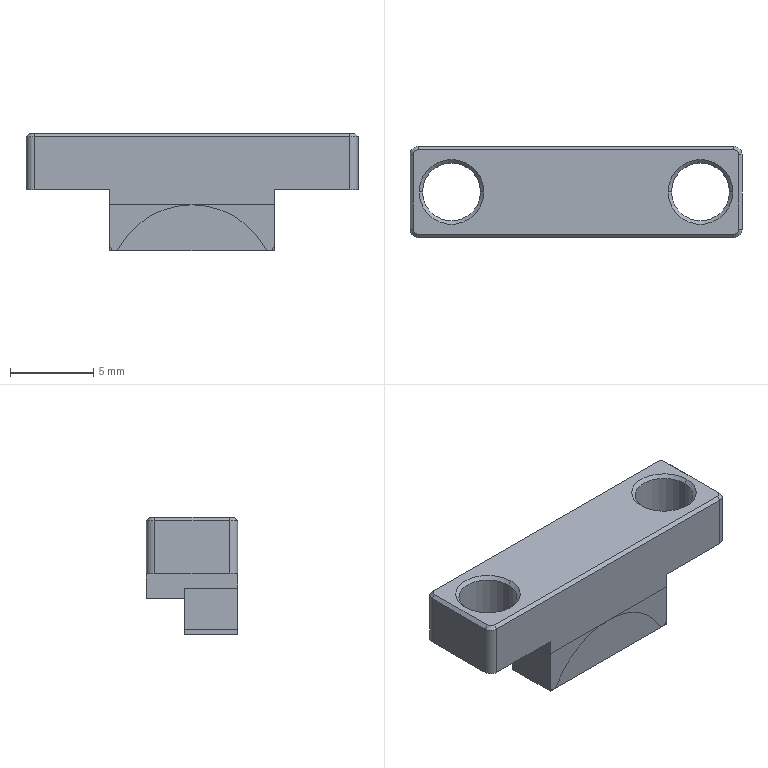NC program | NX | posted with a generic post | part box 20 x 5.5 x 7.057 mm
Whole program:
N10 G17 G21 G94 G90
(FLOOR_WALL_COPY_COPY , TOOL : D63)
N12 T03 M6
N14 G54
N16 G17 G0 G90 X44.499 Y0. B0. C0. S6500 M3
N18 G43 Z30. H3
N20 Z5.
N22 G94 G1 Z2. F1250.
N24 X41.499
N26 X-41.499
N28 X-44.499
N30 Z5.
N32 G0 Z30.
N34 X44.499
N36 Z4.
N38 G1 Z1.
N40 X41.499
N42 X-41.499
N44 X-44.499
N46 Z4.
N48 G0 Z30.
N50 X44.499
N52 Z3.
N54 G1 Z0.
N56 X41.499
N58 X-41.499
N60 X-44.499
N62 Z3.
N64 G0 Z30.
N66 M5
(FLOOR_WALL , TOOL : D6JING)
N68 T16 M6
N70 G54
N72 G17 G0 G90 X2.078 Y-8.75 B0. C0. S9500 M3
N74 G43 Z30. H16
N76 Z-0.377
N78 G94 G1 X0.52 Y-6.05 F1000.
N80 G3 X0. Y-5.75 R0.6
N82 G1 X-9.5 F2500.
N84 G2 X-13. Y-2.25 R3.5
N86 G1 Y2.25
N88 G2 X-9.5 Y5.75 R3.5
N90 G1 X-8.05
N92 Y-3.55
N94 X8.05
N96 Y5.75
N98 X9.5
N100 G2 X13. Y2.25 R3.5
N102 G1 Y-2.25
N104 G2 X9.5 Y-5.75 R3.5
N106 G1 X0.
N108 G3 X-0.52 Y-6.05 R0.6
N110 G1 X-2.078 Y-8.75
N112 G0 X2.078 Z-0.797
N114 G1 X0.52 Y-6.05 F1000.
N116 G3 X0. Y-5.75 R0.6
N118 G1 X-9.5 F2500.
N120 G2 X-13. Y-2.25 R3.5
N122 G1 Y2.25
N124 G2 X-9.5 Y5.75 R3.5
N126 G1 X-8.05
N128 Y-3.55
N130 X8.05
N132 Y5.75
N134 X9.5
N136 G2 X13. Y2.25 R3.5
N138 G1 Y-2.25
N140 G2 X9.5 Y-5.75 R3.5
N142 G1 X0.
N144 G3 X-0.52 Y-6.05 R0.6
N146 G1 X-2.078 Y-8.75
N148 G0 X2.078 Z-1.217
N150 G1 X0.52 Y-6.05 F1000.
N152 G3 X0. Y-5.75 R0.6
N154 G1 X-9.5 F2500.
N156 G2 X-13. Y-2.25 R3.5
N158 G1 Y2.25
N160 G2 X-9.5 Y5.75 R3.5
N162 G1 X-8.05
N164 Y-3.55
N166 X8.05
N168 Y5.75
N170 X9.5
N172 G2 X13. Y2.25 R3.5
N174 G1 Y-2.25
N176 G2 X9.5 Y-5.75 R3.5
N178 G1 X0.
N180 G3 X-0.52 Y-6.05 R0.6
N182 G1 X-2.078 Y-8.75
N184 G0 X2.078 Z-1.637
N186 G1 X0.52 Y-6.05 F1000.
N188 G3 X0. Y-5.75 R0.6
N190 G1 X-9.5 F2500.
N192 G2 X-13. Y-2.25 R3.5
N194 G1 Y2.25
N196 G2 X-9.5 Y5.75 R3.5
N198 G1 X-8.05
N200 Y-3.55
N202 X8.05
N204 Y5.75
N206 X9.5
N208 G2 X13. Y2.25 R3.5
N210 G1 Y-2.25
N212 G2 X9.5 Y-5.75 R3.5
N214 G1 X0.
N216 G3 X-0.52 Y-6.05 R0.6
N218 G1 X-2.078 Y-8.75
N220 G0 X2.078 Z-2.057
N222 G1 X0.52 Y-6.05 F1000.
N224 G3 X0. Y-5.75 R0.6
N226 G1 X-9.5 F2500.
N228 G2 X-13. Y-2.25 R3.5
N230 G1 Y2.25
N232 G2 X-9.5 Y5.75 R3.5
N234 G1 X-8.05
N236 Y-3.55
N238 X8.05
N240 Y5.75
N242 X9.5
N244 G2 X13. Y2.25 R3.5
N246 G1 Y-2.25
N248 G2 X9.5 Y-5.75 R3.5
N250 G1 X0.
N252 G3 X-0.52 Y-6.05 R0.6
N254 G1 X-2.078 Y-8.75
N256 G0 Z30.
N258 X-16. Y-2.078
N260 Z-2.557
N262 G1 X-13.3 Y-0.52 F1000.
N264 G3 X-13. Y0. R0.6
N266 G1 Y2.25 F2500.
N268 G2 X-9.5 Y5.75 R3.5
N270 G1 X-8.05
N272 Y-5.75
N274 X-9.5
N276 G2 X-13. Y-2.25 R3.5
N278 G1 Y0.
N280 G3 X-13.3 Y0.52 R0.6
N282 G1 X-16. Y2.078
N284 G0 Y-2.078 Z-3.057
N286 G1 X-13.3 Y-0.52 F1000.
N288 G3 X-13. Y0. R0.6
N290 G1 Y2.25 F2500.
N292 G2 X-9.5 Y5.75 R3.5
N294 G1 X-8.05
N296 Y-5.75
N298 X-9.5
N300 G2 X-13. Y-2.25 R3.5
N302 G1 Y0.
N304 G3 X-13.3 Y0.52 R0.6
N306 G1 X-16. Y2.078
N308 G0 Y-2.078 Z-3.557
N310 G1 X-13.3 Y-0.52 F1000.
N312 G3 X-13. Y0. R0.6
N314 G1 Y2.25 F2500.
N316 G2 X-9.5 Y5.75 R3.5
N318 G1 X-8.05
N320 Y-5.75
N322 X-9.5
N324 G2 X-13. Y-2.25 R3.5
N326 G1 Y0.
N328 G3 X-13.3 Y0.52 R0.6
N330 G1 X-16. Y2.078
N332 G0 Z30.
N334 X16.
N336 Z-2.557
N338 G1 X13.3 Y0.52 F1000.
N340 G3 X13. Y0. R0.6
N342 G1 Y-2.25 F2500.
N344 G2 X9.5 Y-5.75 R3.5
N346 G1 X8.05
N348 Y5.75
N350 X9.5
N352 G2 X13. Y2.25 R3.5
N354 G1 Y0.
N356 G3 X13.3 Y-0.52 R0.6
N358 G1 X16. Y-2.078
N360 G0 Y2.078 Z-3.057
N362 G1 X13.3 Y0.52 F1000.
N364 G3 X13. Y0. R0.6
N366 G1 Y-2.25 F2500.
N368 G2 X9.5 Y-5.75 R3.5
N370 G1 X8.05
N372 Y5.75
N374 X9.5
N376 G2 X13. Y2.25 R3.5
N378 G1 Y0.
N380 G3 X13.3 Y-0.52 R0.6
N382 G1 X16. Y-2.078
N384 G0 Y2.078 Z-3.557
N386 G1 X13.3 Y0.52 F1000.
N388 G3 X13. Y0. R0.6
N390 G1 Y-2.25 F2500.
N392 G2 X9.5 Y-5.75 R3.5
N394 G1 X8.05
N396 Y5.75
N398 X9.5
N400 G2 X13. Y2.25 R3.5
N402 G1 Y0.
N404 G3 X13.3 Y-0.52 R0.6
N406 G1 X16. Y-2.078
N408 G0 Z30.
(FLOOR_WALL_COPY_1 , TOOL : D6JING)
N410 X-14. Y-0.924
N412 Z-2.657
N414 G1 Z-3.657 F1000.
N416 X-13.3 Y-0.52
N418 G3 X-13. Y0. R0.6
N420 G1 Y2.25
N422 G2 X-9.5 Y5.75 R3.5
N424 G1 X-8.25
N426 Y-5.75
N428 X-9.5
N430 G2 X-13. Y-2.25 R3.5
N432 G1 Y0.
N434 G3 X-13.3 Y0.52 R0.6
N436 G1 X-14. Y0.924
N438 Z-2.657
N440 G0 Z-0.557
N442 G1 X-9.082 Y-6.75 F8000.
N444 G0 Z-2.657
N446 G1 Z-3.657 F1000.
N448 X-8.25 Y-6.27
N450 G3 X-7.95 Y-5.75 R0.6
N452 G1 Y5.75
N454 G3 X-8.25 Y6.27 R0.6
N456 G1 X-9.082 Y6.75
N458 Z-2.657
N460 G0 Z30.
N462 X8.701 Y-4.45
N464 Z-1.157
N466 G1 Z-2.157
N468 X8.47 Y-4.05
N470 G3 X7.95 Y-3.75 R0.6
N472 G1 X-7.95
N474 G3 X-8.47 Y-4.05 R0.6
N476 G1 X-8.701 Y-4.45
N478 Z-1.157
N480 G0 Z0.943
N482 G1 X8.95 Y-4.582 F8000.
N484 G0 Z-1.157
N486 G1 Z-2.157 F1000.
N488 X8.47 Y-3.75
N490 G3 X7.95 Y-3.45 R0.6
N492 G1 X-7.95
N494 G3 X-8.47 Y-3.75 R0.6
N496 G1 X-8.95 Y-4.582
N498 Z-1.157
N500 G0 Z30.
N502 X14. Y0.924
N504 Z-2.657
N506 G1 Z-3.657
N508 X13.3 Y0.52
N510 G3 X13. Y0. R0.6
N512 G1 Y-2.25
N514 G2 X9.5 Y-5.75 R3.5
N516 G1 X8.25
N518 Y5.75
N520 X9.5
N522 G2 X13. Y2.25 R3.5
N524 G1 Y0.
N526 G3 X13.3 Y-0.52 R0.6
N528 G1 X14. Y-0.924
N530 Z-2.657
N532 G0 Z-0.557
N534 G1 X9.082 Y6.75 F8000.
N536 G0 Z-2.657
N538 G1 Z-3.657 F1000.
N540 X8.25 Y6.27
N542 G3 X7.95 Y5.75 R0.6
N544 G1 Y-5.75
N546 G3 X8.25 Y-6.27 R0.6
N548 G1 X9.082 Y-6.75
N550 Z-2.657
N552 G0 Z30.
N554 M5
N556 M2